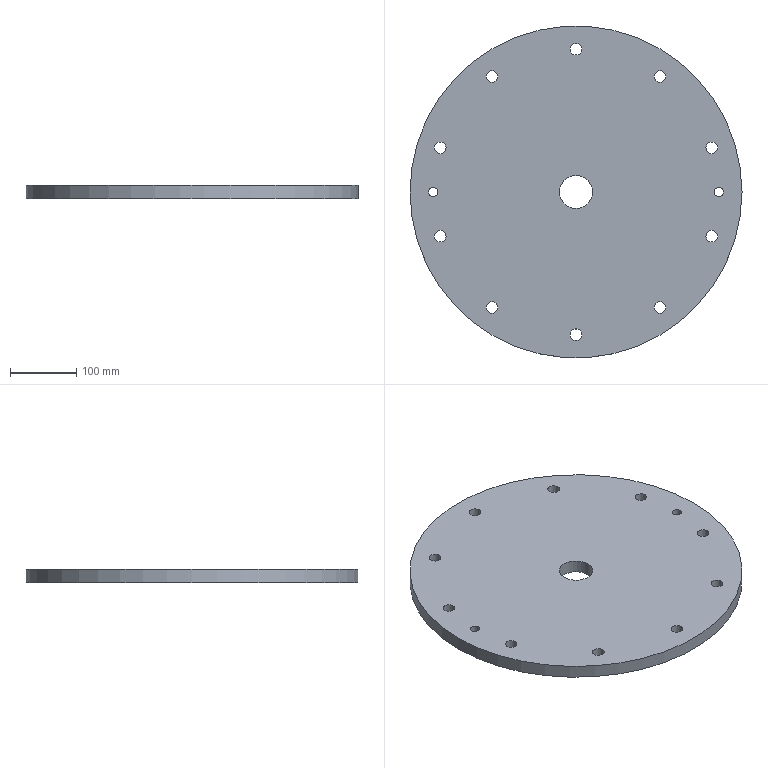CAM job | NX | drilling | part box 500 x 500 x 20 mm | stock box 500 x 500 x 20 mm
Tools:
number,name,description,diameter,corner_radius,flute_length,length,flutes
2,ZXZ,Milling Tool-5 Parameters,6.0,0.0,50.0,75.0,2
17,17.5ZT,Drilling Tool,17.5,0.0,35.0,50.0,2
14,14.0ZT,Drilling Tool,14.0,0.0,35.0,50.0,2
Operations:
program,operation,operation_type,tool,method,geometry_group,spindle_rpm,surface_speed,feed_per_tooth,feed_cut,feed_plunge,cut_length_mm,path_length_mm,cut_time_min,machine_time_min
10-HOLE,DRILLING,Operation,ZXZ,METHOD,A,3500.0,65.0,0.0357,250.0,0.0,60.0,1412.713,0.24,0.3753
10-HOLE,DRILLING_COPY,Operation,17.5ZT,METHOD,A,500.0,27.0,0.1,100.0,0.0,297.575,1878.351,2.976,3.134
10-HOLE,DRILLING_COPY_COPY,Operation,14.0ZT,METHOD,A,700.0,30.0,0.0714,100.0,0.0,57.412,607.835,0.5741,0.6292